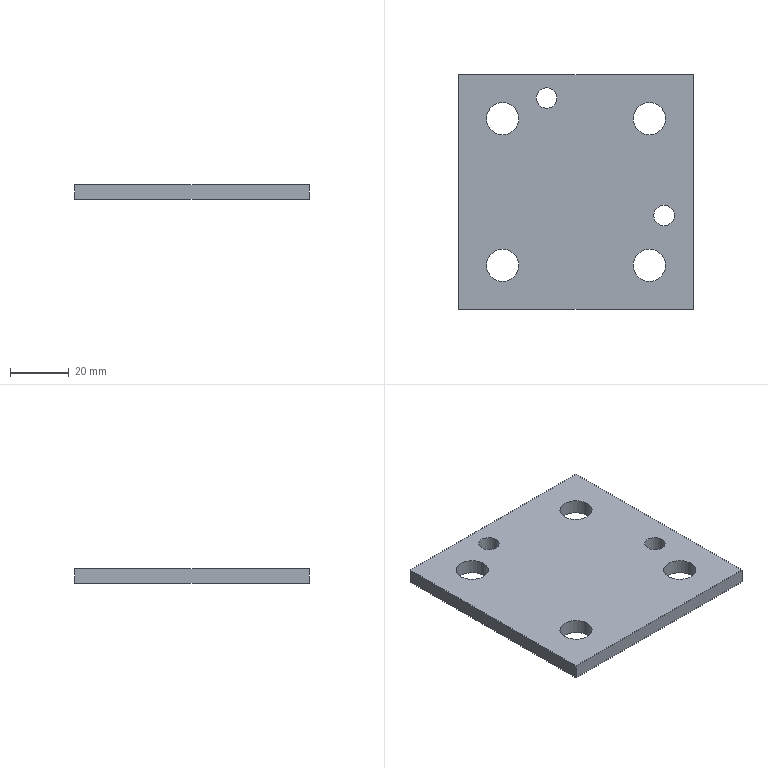Part | NX | features solid 2 | 1 solid | 12 faces | box 80 x 80 x 5 mm | volume 29714 mm3 | plane 6 | cylinder 6 | commonest cylinder face diameters 11 x4 7 x2
STEP:
#1=CARTESIAN_POINT('',(-710.,-45.,93.));
#2=VERTEX_POINT('',#1);
#3=CARTESIAN_POINT('',(-630.,-45.,93.));
#4=VERTEX_POINT('',#3);
#5=CARTESIAN_POINT('',(-720.,-45.,93.));
#6=DIRECTION('',(1.,0.,0.));
#7=VECTOR('',#6,1000.);
#8=LINE('',#5,#7);
#9=EDGE_CURVE('',#2,#4,#8,.T.);
#10=ORIENTED_EDGE('',*,*,#9,.F.);
#11=CARTESIAN_POINT('',(-710.,-45.,88.));
#12=VERTEX_POINT('',#11);
#13=CARTESIAN_POINT('',(-710.,-45.,88.));
#14=DIRECTION('',(0.,0.,1.));
#15=VECTOR('',#14,1000.);
#16=LINE('',#13,#15);
#17=EDGE_CURVE('',#12,#2,#16,.T.);
#18=ORIENTED_EDGE('',*,*,#17,.F.);
#19=CARTESIAN_POINT('',(-630.,-45.,88.));
#20=VERTEX_POINT('',#19);
#21=CARTESIAN_POINT('',(-720.,-45.,88.));
#22=DIRECTION('',(1.,0.,0.));
#23=VECTOR('',#22,1000.);
#24=LINE('',#21,#23);
#25=EDGE_CURVE('',#12,#20,#24,.T.);
#26=ORIENTED_EDGE('',*,*,#25,.T.);
#27=CARTESIAN_POINT('',(-630.,-45.,88.));
#28=DIRECTION('',(0.,0.,1.));
#29=VECTOR('',#28,1000.);
#30=LINE('',#27,#29);
#31=EDGE_CURVE('',#20,#4,#30,.T.);
#32=ORIENTED_EDGE('',*,*,#31,.T.);
#33=EDGE_LOOP('',(#10,#18,#26,#32));
#34=FACE_BOUND('',#33,.T.);
#35=CARTESIAN_POINT('',(-720.,-45.,88.));
#36=DIRECTION('',(0.,1.,0.));
#37=DIRECTION('',(0.,0.,1.));
#38=AXIS2_PLACEMENT_3D('',#35,#36,#37);
#39=PLANE('',#38);
#40=ADVANCED_FACE('',(#34),#39,.F.);
#41=CARTESIAN_POINT('',(-710.,35.,93.));
#42=VERTEX_POINT('',#41);
#43=CARTESIAN_POINT('',(-710.,25.,93.));
#44=DIRECTION('',(0.,-1.,0.));
#45=VECTOR('',#44,1000.);
#46=LINE('',#43,#45);
#47=EDGE_CURVE('',#42,#2,#46,.T.);
#48=ORIENTED_EDGE('',*,*,#47,.F.);
#49=CARTESIAN_POINT('',(-710.,35.,88.));
#50=VERTEX_POINT('',#49);
#51=CARTESIAN_POINT('',(-710.,35.,88.));
#52=DIRECTION('',(0.,0.,1.));
#53=VECTOR('',#52,1000.);
#54=LINE('',#51,#53);
#55=EDGE_CURVE('',#50,#42,#54,.T.);
#56=ORIENTED_EDGE('',*,*,#55,.F.);
#57=CARTESIAN_POINT('',(-710.,25.,88.));
#58=DIRECTION('',(0.,-1.,0.));
#59=VECTOR('',#58,1000.);
#60=LINE('',#57,#59);
#61=EDGE_CURVE('',#50,#12,#60,.T.);
#62=ORIENTED_EDGE('',*,*,#61,.T.);
#63=ORIENTED_EDGE('',*,*,#17,.T.);
#64=EDGE_LOOP('',(#48,#56,#62,#63));
#65=FACE_BOUND('',#64,.T.);
#66=CARTESIAN_POINT('',(-710.,25.,88.));
#67=DIRECTION('',(1.,0.,0.));
#68=DIRECTION('',(0.,0.,1.));
#69=AXIS2_PLACEMENT_3D('',#66,#67,#68);
#70=PLANE('',#69);
#71=ADVANCED_FACE('',(#65),#70,.F.);
#72=CARTESIAN_POINT('',(-630.,35.,93.));
#73=VERTEX_POINT('',#72);
#74=CARTESIAN_POINT('',(-720.,35.,93.));
#75=DIRECTION('',(-1.,0.,0.));
#76=VECTOR('',#75,1000.);
#77=LINE('',#74,#76);
#78=EDGE_CURVE('',#73,#42,#77,.T.);
#79=ORIENTED_EDGE('',*,*,#78,.F.);
#80=CARTESIAN_POINT('',(-630.,35.,88.));
#81=VERTEX_POINT('',#80);
#82=CARTESIAN_POINT('',(-630.,35.,88.));
#83=DIRECTION('',(0.,0.,1.));
#84=VECTOR('',#83,1000.);
#85=LINE('',#82,#84);
#86=EDGE_CURVE('',#81,#73,#85,.T.);
#87=ORIENTED_EDGE('',*,*,#86,.F.);
#88=CARTESIAN_POINT('',(-720.,35.,88.));
#89=DIRECTION('',(-1.,0.,0.));
#90=VECTOR('',#89,1000.);
#91=LINE('',#88,#90);
#92=EDGE_CURVE('',#81,#50,#91,.T.);
#93=ORIENTED_EDGE('',*,*,#92,.T.);
#94=ORIENTED_EDGE('',*,*,#55,.T.);
#95=EDGE_LOOP('',(#79,#87,#93,#94));
#96=FACE_BOUND('',#95,.T.);
#97=CARTESIAN_POINT('',(-720.,35.,88.));
#98=DIRECTION('',(0.,-1.,0.));
#99=DIRECTION('',(0.,0.,-1.));
#100=AXIS2_PLACEMENT_3D('',#97,#98,#99);
#101=PLANE('',#100);
#102=ADVANCED_FACE('',(#96),#101,.F.);
#103=CARTESIAN_POINT('',(-630.,25.,93.));
#104=DIRECTION('',(0.,1.,0.));
#105=VECTOR('',#104,1000.);
#106=LINE('',#103,#105);
#107=EDGE_CURVE('',#4,#73,#106,.T.);
#108=ORIENTED_EDGE('',*,*,#107,.F.);
#109=ORIENTED_EDGE('',*,*,#31,.F.);
#110=CARTESIAN_POINT('',(-630.,25.,88.));
#111=DIRECTION('',(0.,1.,0.));
#112=VECTOR('',#111,1000.);
#113=LINE('',#110,#112);
#114=EDGE_CURVE('',#20,#81,#113,.T.);
#115=ORIENTED_EDGE('',*,*,#114,.T.);
#116=ORIENTED_EDGE('',*,*,#86,.T.);
#117=EDGE_LOOP('',(#108,#109,#115,#116));
#118=FACE_BOUND('',#117,.T.);
#119=CARTESIAN_POINT('',(-630.,25.,88.));
#120=DIRECTION('',(-1.,0.,0.));
#121=DIRECTION('',(0.,0.,-1.));
#122=AXIS2_PLACEMENT_3D('',#119,#120,#121);
#123=PLANE('',#122);
#124=ADVANCED_FACE('',(#118),#123,.F.);
#125=CARTESIAN_POINT('',(-683.5,27.,88.));
#126=VERTEX_POINT('',#125);
#127=CARTESIAN_POINT('',(-680.,27.,88.));
#128=DIRECTION('',(0.,0.,-1.));
#129=DIRECTION('',(-1.,0.,0.));
#130=AXIS2_PLACEMENT_3D('',#127,#128,#129);
#131=CIRCLE('',#130,3.5);
#132=EDGE_CURVE('',#126,#126,#131,.T.);
#133=ORIENTED_EDGE('',*,*,#132,.T.);
#134=EDGE_LOOP('',(#133));
#135=FACE_BOUND('',#134,.T.);
#136=CARTESIAN_POINT('',(-683.5,27.,93.));
#137=VERTEX_POINT('',#136);
#138=CARTESIAN_POINT('',(-680.,27.,93.));
#139=DIRECTION('',(0.,0.,-1.));
#140=DIRECTION('',(-1.,0.,0.));
#141=AXIS2_PLACEMENT_3D('',#138,#139,#140);
#142=CIRCLE('',#141,3.5);
#143=EDGE_CURVE('',#137,#137,#142,.T.);
#144=ORIENTED_EDGE('',*,*,#143,.F.);
#145=EDGE_LOOP('',(#144));
#146=FACE_BOUND('',#145,.T.);
#147=CARTESIAN_POINT('',(-680.,27.,88.));
#148=DIRECTION('',(0.,0.,1.));
#149=DIRECTION('',(-1.,0.,0.));
#150=AXIS2_PLACEMENT_3D('',#147,#148,#149);
#151=CYLINDRICAL_SURFACE('',#150,3.5);
#152=ADVANCED_FACE('',(#135,#146),#151,.F.);
#153=CARTESIAN_POINT('',(-643.5,-13.,88.));
#154=VERTEX_POINT('',#153);
#155=CARTESIAN_POINT('',(-640.,-13.,88.));
#156=DIRECTION('',(0.,0.,-1.));
#157=DIRECTION('',(-1.,0.,0.));
#158=AXIS2_PLACEMENT_3D('',#155,#156,#157);
#159=CIRCLE('',#158,3.5);
#160=EDGE_CURVE('',#154,#154,#159,.T.);
#161=ORIENTED_EDGE('',*,*,#160,.T.);
#162=EDGE_LOOP('',(#161));
#163=FACE_BOUND('',#162,.T.);
#164=CARTESIAN_POINT('',(-643.5,-13.,93.));
#165=VERTEX_POINT('',#164);
#166=CARTESIAN_POINT('',(-640.,-13.,93.));
#167=DIRECTION('',(0.,0.,-1.));
#168=DIRECTION('',(-1.,0.,0.));
#169=AXIS2_PLACEMENT_3D('',#166,#167,#168);
#170=CIRCLE('',#169,3.5);
#171=EDGE_CURVE('',#165,#165,#170,.T.);
#172=ORIENTED_EDGE('',*,*,#171,.F.);
#173=EDGE_LOOP('',(#172));
#174=FACE_BOUND('',#173,.T.);
#175=CARTESIAN_POINT('',(-640.,-13.,88.));
#176=DIRECTION('',(0.,0.,1.));
#177=DIRECTION('',(-1.,0.,0.));
#178=AXIS2_PLACEMENT_3D('',#175,#176,#177);
#179=CYLINDRICAL_SURFACE('',#178,3.5);
#180=ADVANCED_FACE('',(#163,#174),#179,.F.);
#181=CARTESIAN_POINT('',(-650.5,-30.,88.));
#182=VERTEX_POINT('',#181);
#183=CARTESIAN_POINT('',(-645.,-30.,88.));
#184=DIRECTION('',(0.,0.,-1.));
#185=DIRECTION('',(-1.,0.,0.));
#186=AXIS2_PLACEMENT_3D('',#183,#184,#185);
#187=CIRCLE('',#186,5.5);
#188=EDGE_CURVE('',#182,#182,#187,.T.);
#189=ORIENTED_EDGE('',*,*,#188,.T.);
#190=EDGE_LOOP('',(#189));
#191=FACE_BOUND('',#190,.T.);
#192=CARTESIAN_POINT('',(-650.5,-30.,93.));
#193=VERTEX_POINT('',#192);
#194=CARTESIAN_POINT('',(-645.,-30.,93.));
#195=DIRECTION('',(0.,0.,-1.));
#196=DIRECTION('',(-1.,0.,0.));
#197=AXIS2_PLACEMENT_3D('',#194,#195,#196);
#198=CIRCLE('',#197,5.5);
#199=EDGE_CURVE('',#193,#193,#198,.T.);
#200=ORIENTED_EDGE('',*,*,#199,.F.);
#201=EDGE_LOOP('',(#200));
#202=FACE_BOUND('',#201,.T.);
#203=CARTESIAN_POINT('',(-645.,-30.,88.));
#204=DIRECTION('',(0.,0.,1.));
#205=DIRECTION('',(-1.,0.,0.));
#206=AXIS2_PLACEMENT_3D('',#203,#204,#205);
#207=CYLINDRICAL_SURFACE('',#206,5.5);
#208=ADVANCED_FACE('',(#191,#202),#207,.F.);
#209=CARTESIAN_POINT('',(-650.5,20.,88.));
#210=VERTEX_POINT('',#209);
#211=CARTESIAN_POINT('',(-645.,20.,88.));
#212=DIRECTION('',(0.,0.,-1.));
#213=DIRECTION('',(-1.,0.,0.));
#214=AXIS2_PLACEMENT_3D('',#211,#212,#213);
#215=CIRCLE('',#214,5.5);
#216=EDGE_CURVE('',#210,#210,#215,.T.);
#217=ORIENTED_EDGE('',*,*,#216,.T.);
#218=EDGE_LOOP('',(#217));
#219=FACE_BOUND('',#218,.T.);
#220=CARTESIAN_POINT('',(-650.5,20.,93.));
#221=VERTEX_POINT('',#220);
#222=CARTESIAN_POINT('',(-645.,20.,93.));
#223=DIRECTION('',(0.,0.,-1.));
#224=DIRECTION('',(-1.,0.,0.));
#225=AXIS2_PLACEMENT_3D('',#222,#223,#224);
#226=CIRCLE('',#225,5.5);
#227=EDGE_CURVE('',#221,#221,#226,.T.);
#228=ORIENTED_EDGE('',*,*,#227,.F.);
#229=EDGE_LOOP('',(#228));
#230=FACE_BOUND('',#229,.T.);
#231=CARTESIAN_POINT('',(-645.,20.,88.));
#232=DIRECTION('',(0.,0.,1.));
#233=DIRECTION('',(-1.,0.,0.));
#234=AXIS2_PLACEMENT_3D('',#231,#232,#233);
#235=CYLINDRICAL_SURFACE('',#234,5.5);
#236=ADVANCED_FACE('',(#219,#230),#235,.F.);
#237=CARTESIAN_POINT('',(-700.5,20.,88.));
#238=VERTEX_POINT('',#237);
#239=CARTESIAN_POINT('',(-695.,20.,88.));
#240=DIRECTION('',(0.,0.,-1.));
#241=DIRECTION('',(-1.,0.,0.));
#242=AXIS2_PLACEMENT_3D('',#239,#240,#241);
#243=CIRCLE('',#242,5.5);
#244=EDGE_CURVE('',#238,#238,#243,.T.);
#245=ORIENTED_EDGE('',*,*,#244,.T.);
#246=EDGE_LOOP('',(#245));
#247=FACE_BOUND('',#246,.T.);
#248=CARTESIAN_POINT('',(-700.5,20.,93.));
#249=VERTEX_POINT('',#248);
#250=CARTESIAN_POINT('',(-695.,20.,93.));
#251=DIRECTION('',(0.,0.,-1.));
#252=DIRECTION('',(-1.,0.,0.));
#253=AXIS2_PLACEMENT_3D('',#250,#251,#252);
#254=CIRCLE('',#253,5.5);
#255=EDGE_CURVE('',#249,#249,#254,.T.);
#256=ORIENTED_EDGE('',*,*,#255,.F.);
#257=EDGE_LOOP('',(#256));
#258=FACE_BOUND('',#257,.T.);
#259=CARTESIAN_POINT('',(-695.,20.,88.));
#260=DIRECTION('',(0.,0.,1.));
#261=DIRECTION('',(-1.,0.,0.));
#262=AXIS2_PLACEMENT_3D('',#259,#260,#261);
#263=CYLINDRICAL_SURFACE('',#262,5.5);
#264=ADVANCED_FACE('',(#247,#258),#263,.F.);
#265=CARTESIAN_POINT('',(-700.5,-30.,88.));
#266=VERTEX_POINT('',#265);
#267=CARTESIAN_POINT('',(-695.,-30.,88.));
#268=DIRECTION('',(0.,0.,-1.));
#269=DIRECTION('',(-1.,0.,0.));
#270=AXIS2_PLACEMENT_3D('',#267,#268,#269);
#271=CIRCLE('',#270,5.5);
#272=EDGE_CURVE('',#266,#266,#271,.T.);
#273=ORIENTED_EDGE('',*,*,#272,.T.);
#274=EDGE_LOOP('',(#273));
#275=FACE_BOUND('',#274,.T.);
#276=CARTESIAN_POINT('',(-700.5,-30.,93.));
#277=VERTEX_POINT('',#276);
#278=CARTESIAN_POINT('',(-695.,-30.,93.));
#279=DIRECTION('',(0.,0.,-1.));
#280=DIRECTION('',(-1.,0.,0.));
#281=AXIS2_PLACEMENT_3D('',#278,#279,#280);
#282=CIRCLE('',#281,5.5);
#283=EDGE_CURVE('',#277,#277,#282,.T.);
#284=ORIENTED_EDGE('',*,*,#283,.F.);
#285=EDGE_LOOP('',(#284));
#286=FACE_BOUND('',#285,.T.);
#287=CARTESIAN_POINT('',(-695.,-30.,88.));
#288=DIRECTION('',(0.,0.,1.));
#289=DIRECTION('',(-1.,0.,0.));
#290=AXIS2_PLACEMENT_3D('',#287,#288,#289);
#291=CYLINDRICAL_SURFACE('',#290,5.5);
#292=ADVANCED_FACE('',(#275,#286),#291,.F.);
#293=ORIENTED_EDGE('',*,*,#272,.F.);
#294=EDGE_LOOP('',(#293));
#295=FACE_BOUND('',#294,.T.);
#296=ORIENTED_EDGE('',*,*,#244,.F.);
#297=EDGE_LOOP('',(#296));
#298=FACE_BOUND('',#297,.T.);
#299=ORIENTED_EDGE('',*,*,#216,.F.);
#300=EDGE_LOOP('',(#299));
#301=FACE_BOUND('',#300,.T.);
#302=ORIENTED_EDGE('',*,*,#188,.F.);
#303=EDGE_LOOP('',(#302));
#304=FACE_BOUND('',#303,.T.);
#305=ORIENTED_EDGE('',*,*,#160,.F.);
#306=EDGE_LOOP('',(#305));
#307=FACE_BOUND('',#306,.T.);
#308=ORIENTED_EDGE('',*,*,#132,.F.);
#309=EDGE_LOOP('',(#308));
#310=FACE_BOUND('',#309,.T.);
#311=ORIENTED_EDGE('',*,*,#25,.F.);
#312=ORIENTED_EDGE('',*,*,#61,.F.);
#313=ORIENTED_EDGE('',*,*,#92,.F.);
#314=ORIENTED_EDGE('',*,*,#114,.F.);
#315=EDGE_LOOP('',(#311,#312,#313,#314));
#316=FACE_BOUND('',#315,.T.);
#317=CARTESIAN_POINT('',(-720.,25.,88.));
#318=DIRECTION('',(0.,0.,1.));
#319=DIRECTION('',(-1.,0.,0.));
#320=AXIS2_PLACEMENT_3D('',#317,#318,#319);
#321=PLANE('',#320);
#322=ADVANCED_FACE('',(#295,#298,#301,#304,#307,#310,#316),#321,.F.);
#323=ORIENTED_EDGE('',*,*,#283,.T.);
#324=EDGE_LOOP('',(#323));
#325=FACE_BOUND('',#324,.T.);
#326=ORIENTED_EDGE('',*,*,#255,.T.);
#327=EDGE_LOOP('',(#326));
#328=FACE_BOUND('',#327,.T.);
#329=ORIENTED_EDGE('',*,*,#227,.T.);
#330=EDGE_LOOP('',(#329));
#331=FACE_BOUND('',#330,.T.);
#332=ORIENTED_EDGE('',*,*,#199,.T.);
#333=EDGE_LOOP('',(#332));
#334=FACE_BOUND('',#333,.T.);
#335=ORIENTED_EDGE('',*,*,#171,.T.);
#336=EDGE_LOOP('',(#335));
#337=FACE_BOUND('',#336,.T.);
#338=ORIENTED_EDGE('',*,*,#143,.T.);
#339=EDGE_LOOP('',(#338));
#340=FACE_BOUND('',#339,.T.);
#341=ORIENTED_EDGE('',*,*,#9,.T.);
#342=ORIENTED_EDGE('',*,*,#107,.T.);
#343=ORIENTED_EDGE('',*,*,#78,.T.);
#344=ORIENTED_EDGE('',*,*,#47,.T.);
#345=EDGE_LOOP('',(#341,#342,#343,#344));
#346=FACE_BOUND('',#345,.T.);
#347=CARTESIAN_POINT('',(-720.,25.,93.));
#348=DIRECTION('',(0.,0.,1.));
#349=DIRECTION('',(-1.,0.,0.));
#350=AXIS2_PLACEMENT_3D('',#347,#348,#349);
#351=PLANE('',#350);
#352=ADVANCED_FACE('',(#325,#328,#331,#334,#337,#340,#346),#351,.T.);
#353=CLOSED_SHELL('',(#40,#71,#102,#124,#152,#180,#208,#236,#264,#292,#322,#352));
#354=MANIFOLD_SOLID_BREP('',#353);
#355=(LENGTH_UNIT()NAMED_UNIT(*)SI_UNIT(.MILLI.,.METRE.));
#356=UNCERTAINTY_MEASURE_WITH_UNIT(LENGTH_MEASURE(0.00001),#355,'','');
#357=(NAMED_UNIT(*)PLANE_ANGLE_UNIT()SI_UNIT($,.RADIAN.));
#358=(NAMED_UNIT(*)SI_UNIT($,.STERADIAN.)SOLID_ANGLE_UNIT());
#359=(GEOMETRIC_REPRESENTATION_CONTEXT(3)GLOBAL_UNCERTAINTY_ASSIGNED_CONTEXT((#356))GLOBAL_UNIT_ASSIGNED_CONTEXT((#355,#357,#358))REPRESENTATION_CONTEXT('',''));
#360=ADVANCED_BREP_SHAPE_REPRESENTATION('',(#354),#359);